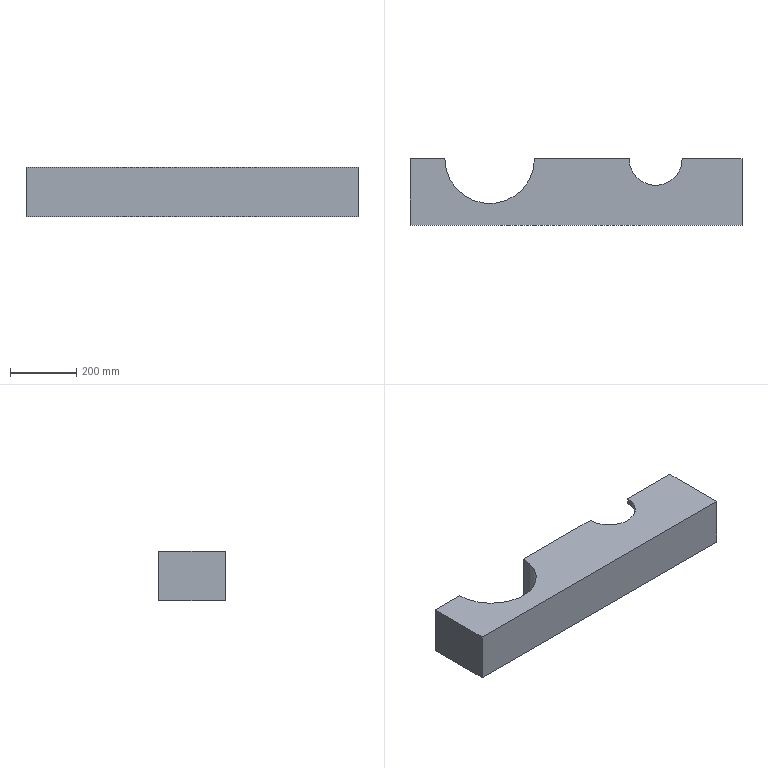Part | SolidWorks | features RefAxis 2, Chamfer 1, Extrusion 1, ICE 1, RevCut 1 | 1 solid | 19 faces | box 1000 x 200 x 150 mm | volume 22425057 mm3 | plane 12 | cylinder 6 | cone 1 | commonest cylinder face diameters 250 x2 160 x1 220 x1 270 x1 280 x1
STEP:
#1=CARTESIAN_POINT('',(660.,0.,150.));
#2=VERTEX_POINT('',#1);
#3=CARTESIAN_POINT('',(660.,0.,132.));
#4=VERTEX_POINT('',#3);
#5=CARTESIAN_POINT('',(660.,0.,0.));
#6=DIRECTION('',(0.,0.,-1.));
#7=VECTOR('',#6,1000.);
#8=LINE('',#5,#7);
#9=EDGE_CURVE('',#2,#4,#8,.T.);
#10=ORIENTED_EDGE('',*,*,#9,.T.);
#11=CARTESIAN_POINT('',(650.,0.,122.));
#12=VERTEX_POINT('',#11);
#13=CARTESIAN_POINT('',(740.,0.,212.));
#14=DIRECTION('',(-0.7071,0.,-0.7071));
#15=VECTOR('',#14,1000.);
#16=LINE('',#13,#15);
#17=EDGE_CURVE('',#4,#12,#16,.T.);
#18=ORIENTED_EDGE('',*,*,#17,.T.);
#19=CARTESIAN_POINT('',(615.,0.,122.));
#20=VERTEX_POINT('',#19);
#21=CARTESIAN_POINT('',(0.,0.,122.));
#22=DIRECTION('',(-1.,0.,0.));
#23=VECTOR('',#22,1000.);
#24=LINE('',#21,#23);
#25=EDGE_CURVE('',#12,#20,#24,.T.);
#26=ORIENTED_EDGE('',*,*,#25,.T.);
#27=CARTESIAN_POINT('',(615.,0.,93.));
#28=VERTEX_POINT('',#27);
#29=CARTESIAN_POINT('',(615.,0.,0.));
#30=DIRECTION('',(0.,0.,-1.));
#31=VECTOR('',#30,1000.);
#32=LINE('',#29,#31);
#33=EDGE_CURVE('',#20,#28,#32,.T.);
#34=ORIENTED_EDGE('',*,*,#33,.T.);
#35=CARTESIAN_POINT('',(600.,0.,93.));
#36=VERTEX_POINT('',#35);
#37=CARTESIAN_POINT('',(0.,0.,93.));
#38=DIRECTION('',(-1.,0.,0.));
#39=VECTOR('',#38,1000.);
#40=LINE('',#37,#39);
#41=EDGE_CURVE('',#28,#36,#40,.T.);
#42=ORIENTED_EDGE('',*,*,#41,.T.);
#43=CARTESIAN_POINT('',(600.,0.,81.));
#44=VERTEX_POINT('',#43);
#45=CARTESIAN_POINT('',(600.,0.,0.));
#46=DIRECTION('',(0.,0.,-1.));
#47=VECTOR('',#46,1000.);
#48=LINE('',#45,#47);
#49=EDGE_CURVE('',#36,#44,#48,.T.);
#50=ORIENTED_EDGE('',*,*,#49,.T.);
#51=CARTESIAN_POINT('',(615.,0.,81.));
#52=VERTEX_POINT('',#51);
#53=CARTESIAN_POINT('',(0.,0.,81.));
#54=DIRECTION('',(1.,0.,0.));
#55=VECTOR('',#54,1000.);
#56=LINE('',#53,#55);
#57=EDGE_CURVE('',#44,#52,#56,.T.);
#58=ORIENTED_EDGE('',*,*,#57,.T.);
#59=CARTESIAN_POINT('',(615.,0.,15.));
#60=VERTEX_POINT('',#59);
#61=CARTESIAN_POINT('',(615.,0.,0.));
#62=DIRECTION('',(0.,0.,-1.));
#63=VECTOR('',#62,1000.);
#64=LINE('',#61,#63);
#65=EDGE_CURVE('',#52,#60,#64,.T.);
#66=ORIENTED_EDGE('',*,*,#65,.T.);
#67=CARTESIAN_POINT('',(630.,0.,15.));
#68=VERTEX_POINT('',#67);
#69=CARTESIAN_POINT('',(0.,0.,15.));
#70=DIRECTION('',(1.,0.,0.));
#71=VECTOR('',#70,1000.);
#72=LINE('',#69,#71);
#73=EDGE_CURVE('',#60,#68,#72,.T.);
#74=ORIENTED_EDGE('',*,*,#73,.T.);
#75=CARTESIAN_POINT('',(630.,0.,0.));
#76=VERTEX_POINT('',#75);
#77=CARTESIAN_POINT('',(630.,0.,0.));
#78=DIRECTION('',(0.,0.,-1.));
#79=VECTOR('',#78,1000.);
#80=LINE('',#77,#79);
#81=EDGE_CURVE('',#68,#76,#80,.T.);
#82=ORIENTED_EDGE('',*,*,#81,.T.);
#83=CARTESIAN_POINT('',(375.,0.,0.));
#84=VERTEX_POINT('',#83);
#85=CARTESIAN_POINT('',(0.,0.,0.));
#86=DIRECTION('',(-1.,0.,0.));
#87=VECTOR('',#86,1000.);
#88=LINE('',#85,#87);
#89=EDGE_CURVE('',#76,#84,#88,.T.);
#90=ORIENTED_EDGE('',*,*,#89,.T.);
#91=CARTESIAN_POINT('',(375.,0.,150.));
#92=VERTEX_POINT('',#91);
#93=CARTESIAN_POINT('',(375.,0.,0.));
#94=DIRECTION('',(0.,0.,1.));
#95=VECTOR('',#94,1000.);
#96=LINE('',#93,#95);
#97=EDGE_CURVE('',#84,#92,#96,.T.);
#98=ORIENTED_EDGE('',*,*,#97,.T.);
#99=CARTESIAN_POINT('',(0.,0.,150.));
#100=DIRECTION('',(-1.,0.,0.));
#101=VECTOR('',#100,1000.);
#102=LINE('',#99,#101);
#103=EDGE_CURVE('',#2,#92,#102,.T.);
#104=ORIENTED_EDGE('',*,*,#103,.F.);
#105=EDGE_LOOP('',(#10,#18,#26,#34,#42,#50,#58,#66,#74,#82,#90,#98,#104));
#106=FACE_OUTER_BOUND('',#105,.T.);
#107=CARTESIAN_POINT('',(0.,0.,150.));
#108=DIRECTION('',(0.,-1.,0.));
#109=DIRECTION('',(0.,0.,-1.));
#110=AXIS2_PLACEMENT_3D('',#107,#108,#109);
#111=PLANE('',#110);
#112=ADVANCED_FACE('',(#106),#111,.F.);
#113=CARTESIAN_POINT('',(865.,0.,122.));
#114=VERTEX_POINT('',#113);
#115=CARTESIAN_POINT('',(830.,0.,122.));
#116=VERTEX_POINT('',#115);
#117=CARTESIAN_POINT('',(0.,0.,122.));
#118=DIRECTION('',(-1.,0.,0.));
#119=VECTOR('',#118,1000.);
#120=LINE('',#117,#119);
#121=EDGE_CURVE('',#114,#116,#120,.T.);
#122=ORIENTED_EDGE('',*,*,#121,.T.);
#123=CARTESIAN_POINT('',(820.,0.,132.));
#124=VERTEX_POINT('',#123);
#125=CARTESIAN_POINT('',(740.,0.,212.));
#126=DIRECTION('',(-0.7071,0.,0.7071));
#127=VECTOR('',#126,1000.);
#128=LINE('',#125,#127);
#129=EDGE_CURVE('',#116,#124,#128,.T.);
#130=ORIENTED_EDGE('',*,*,#129,.T.);
#131=CARTESIAN_POINT('',(820.,0.,150.));
#132=VERTEX_POINT('',#131);
#133=CARTESIAN_POINT('',(820.,0.,0.));
#134=DIRECTION('',(0.,0.,1.));
#135=VECTOR('',#134,1000.);
#136=LINE('',#133,#135);
#137=EDGE_CURVE('',#124,#132,#136,.T.);
#138=ORIENTED_EDGE('',*,*,#137,.T.);
#139=CARTESIAN_POINT('',(1000.,0.,150.));
#140=VERTEX_POINT('',#139);
#141=CARTESIAN_POINT('',(0.,0.,150.));
#142=DIRECTION('',(-1.,0.,0.));
#143=VECTOR('',#142,1000.);
#144=LINE('',#141,#143);
#145=EDGE_CURVE('',#140,#132,#144,.T.);
#146=ORIENTED_EDGE('',*,*,#145,.F.);
#147=CARTESIAN_POINT('',(1000.,0.,0.));
#148=VERTEX_POINT('',#147);
#149=CARTESIAN_POINT('',(1000.,0.,150.));
#150=DIRECTION('',(0.,0.,-1.));
#151=VECTOR('',#150,1000.);
#152=LINE('',#149,#151);
#153=EDGE_CURVE('',#140,#148,#152,.T.);
#154=ORIENTED_EDGE('',*,*,#153,.T.);
#155=CARTESIAN_POINT('',(850.,0.,0.));
#156=VERTEX_POINT('',#155);
#157=CARTESIAN_POINT('',(0.,0.,0.));
#158=DIRECTION('',(-1.,0.,0.));
#159=VECTOR('',#158,1000.);
#160=LINE('',#157,#159);
#161=EDGE_CURVE('',#148,#156,#160,.T.);
#162=ORIENTED_EDGE('',*,*,#161,.T.);
#163=CARTESIAN_POINT('',(850.,0.,15.));
#164=VERTEX_POINT('',#163);
#165=CARTESIAN_POINT('',(850.,0.,0.));
#166=DIRECTION('',(0.,0.,1.));
#167=VECTOR('',#166,1000.);
#168=LINE('',#165,#167);
#169=EDGE_CURVE('',#156,#164,#168,.T.);
#170=ORIENTED_EDGE('',*,*,#169,.T.);
#171=CARTESIAN_POINT('',(865.,0.,15.));
#172=VERTEX_POINT('',#171);
#173=CARTESIAN_POINT('',(0.,0.,15.));
#174=DIRECTION('',(1.,0.,0.));
#175=VECTOR('',#174,1000.);
#176=LINE('',#173,#175);
#177=EDGE_CURVE('',#164,#172,#176,.T.);
#178=ORIENTED_EDGE('',*,*,#177,.T.);
#179=CARTESIAN_POINT('',(865.,0.,81.));
#180=VERTEX_POINT('',#179);
#181=CARTESIAN_POINT('',(865.,0.,0.));
#182=DIRECTION('',(0.,0.,1.));
#183=VECTOR('',#182,1000.);
#184=LINE('',#181,#183);
#185=EDGE_CURVE('',#172,#180,#184,.T.);
#186=ORIENTED_EDGE('',*,*,#185,.T.);
#187=CARTESIAN_POINT('',(880.,0.,81.));
#188=VERTEX_POINT('',#187);
#189=CARTESIAN_POINT('',(0.,0.,81.));
#190=DIRECTION('',(1.,0.,0.));
#191=VECTOR('',#190,1000.);
#192=LINE('',#189,#191);
#193=EDGE_CURVE('',#180,#188,#192,.T.);
#194=ORIENTED_EDGE('',*,*,#193,.T.);
#195=CARTESIAN_POINT('',(880.,0.,93.));
#196=VERTEX_POINT('',#195);
#197=CARTESIAN_POINT('',(880.,0.,0.));
#198=DIRECTION('',(0.,0.,1.));
#199=VECTOR('',#198,1000.);
#200=LINE('',#197,#199);
#201=EDGE_CURVE('',#188,#196,#200,.T.);
#202=ORIENTED_EDGE('',*,*,#201,.T.);
#203=CARTESIAN_POINT('',(865.,0.,93.));
#204=VERTEX_POINT('',#203);
#205=CARTESIAN_POINT('',(0.,0.,93.));
#206=DIRECTION('',(-1.,0.,0.));
#207=VECTOR('',#206,1000.);
#208=LINE('',#205,#207);
#209=EDGE_CURVE('',#196,#204,#208,.T.);
#210=ORIENTED_EDGE('',*,*,#209,.T.);
#211=CARTESIAN_POINT('',(865.,0.,0.));
#212=DIRECTION('',(0.,0.,1.));
#213=VECTOR('',#212,1000.);
#214=LINE('',#211,#213);
#215=EDGE_CURVE('',#204,#114,#214,.T.);
#216=ORIENTED_EDGE('',*,*,#215,.T.);
#217=EDGE_LOOP('',(#122,#130,#138,#146,#154,#162,#170,#178,#186,#194,#202,#210,#216));
#218=FACE_OUTER_BOUND('',#217,.T.);
#219=CARTESIAN_POINT('',(0.,0.,150.));
#220=DIRECTION('',(0.,-1.,0.));
#221=DIRECTION('',(0.,0.,-1.));
#222=AXIS2_PLACEMENT_3D('',#219,#220,#221);
#223=PLANE('',#222);
#224=ADVANCED_FACE('',(#218),#223,.F.);
#225=CARTESIAN_POINT('',(0.,0.,0.));
#226=VERTEX_POINT('',#225);
#227=CARTESIAN_POINT('',(0.,-200.,0.));
#228=VERTEX_POINT('',#227);
#229=CARTESIAN_POINT('',(0.,0.,0.));
#230=DIRECTION('',(0.,-1.,0.));
#231=VECTOR('',#230,1000.);
#232=LINE('',#229,#231);
#233=EDGE_CURVE('',#226,#228,#232,.T.);
#234=ORIENTED_EDGE('',*,*,#233,.T.);
#235=CARTESIAN_POINT('',(0.,-200.,150.));
#236=VERTEX_POINT('',#235);
#237=CARTESIAN_POINT('',(0.,-200.,150.));
#238=DIRECTION('',(0.,0.,-1.));
#239=VECTOR('',#238,1000.);
#240=LINE('',#237,#239);
#241=EDGE_CURVE('',#236,#228,#240,.T.);
#242=ORIENTED_EDGE('',*,*,#241,.F.);
#243=CARTESIAN_POINT('',(0.,0.,150.));
#244=VERTEX_POINT('',#243);
#245=CARTESIAN_POINT('',(0.,0.,150.));
#246=DIRECTION('',(0.,-1.,0.));
#247=VECTOR('',#246,1000.);
#248=LINE('',#245,#247);
#249=EDGE_CURVE('',#244,#236,#248,.T.);
#250=ORIENTED_EDGE('',*,*,#249,.F.);
#251=CARTESIAN_POINT('',(0.,0.,150.));
#252=DIRECTION('',(0.,0.,-1.));
#253=VECTOR('',#252,1000.);
#254=LINE('',#251,#253);
#255=EDGE_CURVE('',#244,#226,#254,.T.);
#256=ORIENTED_EDGE('',*,*,#255,.T.);
#257=EDGE_LOOP('',(#234,#242,#250,#256));
#258=FACE_OUTER_BOUND('',#257,.T.);
#259=CARTESIAN_POINT('',(0.,0.,150.));
#260=DIRECTION('',(1.,0.,0.));
#261=DIRECTION('',(0.,0.,-1.));
#262=AXIS2_PLACEMENT_3D('',#259,#260,#261);
#263=PLANE('',#262);
#264=ADVANCED_FACE('',(#258),#263,.F.);
#265=CARTESIAN_POINT('',(1000.,-200.,0.));
#266=VERTEX_POINT('',#265);
#267=CARTESIAN_POINT('',(0.,-200.,0.));
#268=DIRECTION('',(1.,0.,0.));
#269=VECTOR('',#268,1000.);
#270=LINE('',#267,#269);
#271=EDGE_CURVE('',#228,#266,#270,.T.);
#272=ORIENTED_EDGE('',*,*,#271,.T.);
#273=CARTESIAN_POINT('',(1000.,-200.,150.));
#274=VERTEX_POINT('',#273);
#275=CARTESIAN_POINT('',(1000.,-200.,150.));
#276=DIRECTION('',(0.,0.,-1.));
#277=VECTOR('',#276,1000.);
#278=LINE('',#275,#277);
#279=EDGE_CURVE('',#274,#266,#278,.T.);
#280=ORIENTED_EDGE('',*,*,#279,.F.);
#281=CARTESIAN_POINT('',(0.,-200.,150.));
#282=DIRECTION('',(1.,0.,0.));
#283=VECTOR('',#282,1000.);
#284=LINE('',#281,#283);
#285=EDGE_CURVE('',#236,#274,#284,.T.);
#286=ORIENTED_EDGE('',*,*,#285,.F.);
#287=ORIENTED_EDGE('',*,*,#241,.T.);
#288=EDGE_LOOP('',(#272,#280,#286,#287));
#289=FACE_OUTER_BOUND('',#288,.T.);
#290=CARTESIAN_POINT('',(0.,-200.,150.));
#291=DIRECTION('',(0.,1.,0.));
#292=DIRECTION('',(0.,0.,1.));
#293=AXIS2_PLACEMENT_3D('',#290,#291,#292);
#294=PLANE('',#293);
#295=ADVANCED_FACE('',(#289),#294,.F.);
#296=CARTESIAN_POINT('',(1000.,0.,0.));
#297=DIRECTION('',(0.,1.,0.));
#298=VECTOR('',#297,1000.);
#299=LINE('',#296,#298);
#300=EDGE_CURVE('',#266,#148,#299,.T.);
#301=ORIENTED_EDGE('',*,*,#300,.T.);
#302=ORIENTED_EDGE('',*,*,#153,.F.);
#303=CARTESIAN_POINT('',(1000.,0.,150.));
#304=DIRECTION('',(0.,1.,0.));
#305=VECTOR('',#304,1000.);
#306=LINE('',#303,#305);
#307=EDGE_CURVE('',#274,#140,#306,.T.);
#308=ORIENTED_EDGE('',*,*,#307,.F.);
#309=ORIENTED_EDGE('',*,*,#279,.T.);
#310=EDGE_LOOP('',(#301,#302,#308,#309));
#311=FACE_OUTER_BOUND('',#310,.T.);
#312=CARTESIAN_POINT('',(1000.,0.,150.));
#313=DIRECTION('',(-1.,0.,0.));
#314=DIRECTION('',(0.,0.,1.));
#315=AXIS2_PLACEMENT_3D('',#312,#313,#314);
#316=PLANE('',#315);
#317=ADVANCED_FACE('',(#311),#316,.F.);
#318=CARTESIAN_POINT('',(105.,0.,150.));
#319=VERTEX_POINT('',#318);
#320=CARTESIAN_POINT('',(0.,0.,150.));
#321=DIRECTION('',(-1.,0.,0.));
#322=VECTOR('',#321,1000.);
#323=LINE('',#320,#322);
#324=EDGE_CURVE('',#319,#244,#323,.T.);
#325=ORIENTED_EDGE('',*,*,#324,.F.);
#326=CARTESIAN_POINT('',(105.,0.,0.));
#327=VERTEX_POINT('',#326);
#328=CARTESIAN_POINT('',(105.,0.,0.));
#329=DIRECTION('',(0.,0.,-1.));
#330=VECTOR('',#329,1000.);
#331=LINE('',#328,#330);
#332=EDGE_CURVE('',#319,#327,#331,.T.);
#333=ORIENTED_EDGE('',*,*,#332,.T.);
#334=CARTESIAN_POINT('',(0.,0.,0.));
#335=DIRECTION('',(-1.,0.,0.));
#336=VECTOR('',#335,1000.);
#337=LINE('',#334,#336);
#338=EDGE_CURVE('',#327,#226,#337,.T.);
#339=ORIENTED_EDGE('',*,*,#338,.T.);
#340=ORIENTED_EDGE('',*,*,#255,.F.);
#341=EDGE_LOOP('',(#325,#333,#339,#340));
#342=FACE_OUTER_BOUND('',#341,.T.);
#343=CARTESIAN_POINT('',(0.,0.,150.));
#344=DIRECTION('',(0.,-1.,0.));
#345=DIRECTION('',(0.,0.,-1.));
#346=AXIS2_PLACEMENT_3D('',#343,#344,#345);
#347=PLANE('',#346);
#348=ADVANCED_FACE('',(#342),#347,.F.);
#349=CARTESIAN_POINT('',(240.,0.,150.));
#350=DIRECTION('',(0.,0.,1.));
#351=DIRECTION('',(1.,0.,0.));
#352=AXIS2_PLACEMENT_3D('',#349,#350,#351);
#353=CIRCLE('',#352,135.);
#354=EDGE_CURVE('',#319,#92,#353,.T.);
#355=ORIENTED_EDGE('',*,*,#354,.F.);
#356=ORIENTED_EDGE('',*,*,#324,.T.);
#357=ORIENTED_EDGE('',*,*,#249,.T.);
#358=ORIENTED_EDGE('',*,*,#285,.T.);
#359=ORIENTED_EDGE('',*,*,#307,.T.);
#360=ORIENTED_EDGE('',*,*,#145,.T.);
#361=CARTESIAN_POINT('',(740.,0.,150.));
#362=DIRECTION('',(0.,0.,1.));
#363=DIRECTION('',(1.,0.,0.));
#364=AXIS2_PLACEMENT_3D('',#361,#362,#363);
#365=CIRCLE('',#364,80.);
#366=EDGE_CURVE('',#2,#132,#365,.T.);
#367=ORIENTED_EDGE('',*,*,#366,.F.);
#368=ORIENTED_EDGE('',*,*,#103,.T.);
#369=EDGE_LOOP('',(#355,#356,#357,#358,#359,#360,#367,#368));
#370=FACE_OUTER_BOUND('',#369,.T.);
#371=CARTESIAN_POINT('',(0.,0.,150.));
#372=DIRECTION('',(0.,0.,1.));
#373=DIRECTION('',(1.,0.,0.));
#374=AXIS2_PLACEMENT_3D('',#371,#372,#373);
#375=PLANE('',#374);
#376=ADVANCED_FACE('',(#370),#375,.T.);
#377=ORIENTED_EDGE('',*,*,#89,.F.);
#378=CARTESIAN_POINT('',(740.,0.,0.));
#379=DIRECTION('',(0.,0.,-1.));
#380=DIRECTION('',(-1.,0.,0.));
#381=AXIS2_PLACEMENT_3D('',#378,#379,#380);
#382=CIRCLE('',#381,110.);
#383=EDGE_CURVE('',#156,#76,#382,.T.);
#384=ORIENTED_EDGE('',*,*,#383,.F.);
#385=ORIENTED_EDGE('',*,*,#161,.F.);
#386=ORIENTED_EDGE('',*,*,#300,.F.);
#387=ORIENTED_EDGE('',*,*,#271,.F.);
#388=ORIENTED_EDGE('',*,*,#233,.F.);
#389=ORIENTED_EDGE('',*,*,#338,.F.);
#390=CARTESIAN_POINT('',(240.,0.,0.));
#391=DIRECTION('',(0.,0.,1.));
#392=DIRECTION('',(1.,0.,0.));
#393=AXIS2_PLACEMENT_3D('',#390,#391,#392);
#394=CIRCLE('',#393,135.);
#395=EDGE_CURVE('',#327,#84,#394,.T.);
#396=ORIENTED_EDGE('',*,*,#395,.T.);
#397=EDGE_LOOP('',(#377,#384,#385,#386,#387,#388,#389,#396));
#398=FACE_OUTER_BOUND('',#397,.T.);
#399=CARTESIAN_POINT('',(0.,0.,0.));
#400=DIRECTION('',(0.,0.,1.));
#401=DIRECTION('',(1.,0.,0.));
#402=AXIS2_PLACEMENT_3D('',#399,#400,#401);
#403=PLANE('',#402);
#404=ADVANCED_FACE('',(#398),#403,.F.);
#405=ORIENTED_EDGE('',*,*,#137,.F.);
#406=CARTESIAN_POINT('',(740.,0.,132.));
#407=DIRECTION('',(0.,0.,-1.));
#408=DIRECTION('',(1.,0.,0.));
#409=AXIS2_PLACEMENT_3D('',#406,#407,#408);
#410=CIRCLE('',#409,80.);
#411=EDGE_CURVE('',#124,#4,#410,.T.);
#412=ORIENTED_EDGE('',*,*,#411,.T.);
#413=ORIENTED_EDGE('',*,*,#9,.F.);
#414=ORIENTED_EDGE('',*,*,#366,.T.);
#415=EDGE_LOOP('',(#405,#412,#413,#414));
#416=FACE_OUTER_BOUND('',#415,.T.);
#417=CARTESIAN_POINT('',(740.,0.,0.));
#418=DIRECTION('',(0.,0.,1.));
#419=DIRECTION('',(1.,0.,0.));
#420=AXIS2_PLACEMENT_3D('',#417,#418,#419);
#421=CYLINDRICAL_SURFACE('',#420,80.);
#422=ADVANCED_FACE('',(#416),#421,.F.);
#423=ORIENTED_EDGE('',*,*,#395,.F.);
#424=ORIENTED_EDGE('',*,*,#332,.F.);
#425=ORIENTED_EDGE('',*,*,#354,.T.);
#426=ORIENTED_EDGE('',*,*,#97,.F.);
#427=EDGE_LOOP('',(#423,#424,#425,#426));
#428=FACE_OUTER_BOUND('',#427,.T.);
#429=CARTESIAN_POINT('',(240.,0.,0.));
#430=DIRECTION('',(0.,0.,1.));
#431=DIRECTION('',(1.,0.,0.));
#432=AXIS2_PLACEMENT_3D('',#429,#430,#431);
#433=CYLINDRICAL_SURFACE('',#432,135.);
#434=ADVANCED_FACE('',(#428),#433,.F.);
#435=CARTESIAN_POINT('',(740.,0.,122.));
#436=DIRECTION('',(0.,0.,-1.));
#437=DIRECTION('',(-1.,0.,0.));
#438=AXIS2_PLACEMENT_3D('',#435,#436,#437);
#439=CIRCLE('',#438,125.);
#440=EDGE_CURVE('',#114,#20,#439,.T.);
#441=ORIENTED_EDGE('',*,*,#440,.F.);
#442=ORIENTED_EDGE('',*,*,#215,.F.);
#443=CARTESIAN_POINT('',(740.,0.,93.));
#444=DIRECTION('',(0.,0.,-1.));
#445=DIRECTION('',(-1.,0.,0.));
#446=AXIS2_PLACEMENT_3D('',#443,#444,#445);
#447=CIRCLE('',#446,125.);
#448=EDGE_CURVE('',#204,#28,#447,.T.);
#449=ORIENTED_EDGE('',*,*,#448,.T.);
#450=ORIENTED_EDGE('',*,*,#33,.F.);
#451=EDGE_LOOP('',(#441,#442,#449,#450));
#452=FACE_OUTER_BOUND('',#451,.T.);
#453=CARTESIAN_POINT('',(740.,0.,0.));
#454=DIRECTION('',(0.,0.,-1.));
#455=DIRECTION('',(-1.,0.,0.));
#456=AXIS2_PLACEMENT_3D('',#453,#454,#455);
#457=CYLINDRICAL_SURFACE('',#456,125.);
#458=ADVANCED_FACE('',(#452),#457,.F.);
#459=ORIENTED_EDGE('',*,*,#448,.F.);
#460=ORIENTED_EDGE('',*,*,#209,.F.);
#461=CARTESIAN_POINT('',(740.,0.,93.));
#462=DIRECTION('',(0.,0.,-1.));
#463=DIRECTION('',(-1.,0.,0.));
#464=AXIS2_PLACEMENT_3D('',#461,#462,#463);
#465=CIRCLE('',#464,140.);
#466=EDGE_CURVE('',#196,#36,#465,.T.);
#467=ORIENTED_EDGE('',*,*,#466,.T.);
#468=ORIENTED_EDGE('',*,*,#41,.F.);
#469=EDGE_LOOP('',(#459,#460,#467,#468));
#470=FACE_OUTER_BOUND('',#469,.T.);
#471=CARTESIAN_POINT('',(600.,0.,93.));
#472=DIRECTION('',(0.,0.,1.));
#473=DIRECTION('',(1.,0.,0.));
#474=AXIS2_PLACEMENT_3D('',#471,#472,#473);
#475=PLANE('',#474);
#476=ADVANCED_FACE('',(#470),#475,.F.);
#477=ORIENTED_EDGE('',*,*,#466,.F.);
#478=ORIENTED_EDGE('',*,*,#201,.F.);
#479=CARTESIAN_POINT('',(740.,0.,81.));
#480=DIRECTION('',(0.,0.,-1.));
#481=DIRECTION('',(-1.,0.,0.));
#482=AXIS2_PLACEMENT_3D('',#479,#480,#481);
#483=CIRCLE('',#482,140.);
#484=EDGE_CURVE('',#188,#44,#483,.T.);
#485=ORIENTED_EDGE('',*,*,#484,.T.);
#486=ORIENTED_EDGE('',*,*,#49,.F.);
#487=EDGE_LOOP('',(#477,#478,#485,#486));
#488=FACE_OUTER_BOUND('',#487,.T.);
#489=CARTESIAN_POINT('',(740.,0.,0.));
#490=DIRECTION('',(0.,0.,-1.));
#491=DIRECTION('',(-1.,0.,0.));
#492=AXIS2_PLACEMENT_3D('',#489,#490,#491);
#493=CYLINDRICAL_SURFACE('',#492,140.);
#494=ADVANCED_FACE('',(#488),#493,.F.);
#495=ORIENTED_EDGE('',*,*,#484,.F.);
#496=ORIENTED_EDGE('',*,*,#193,.F.);
#497=CARTESIAN_POINT('',(740.,0.,81.));
#498=DIRECTION('',(0.,0.,-1.));
#499=DIRECTION('',(-1.,0.,0.));
#500=AXIS2_PLACEMENT_3D('',#497,#498,#499);
#501=CIRCLE('',#500,125.);
#502=EDGE_CURVE('',#180,#52,#501,.T.);
#503=ORIENTED_EDGE('',*,*,#502,.T.);
#504=ORIENTED_EDGE('',*,*,#57,.F.);
#505=EDGE_LOOP('',(#495,#496,#503,#504));
#506=FACE_OUTER_BOUND('',#505,.T.);
#507=CARTESIAN_POINT('',(615.,0.,81.));
#508=DIRECTION('',(0.,0.,-1.));
#509=DIRECTION('',(-1.,0.,0.));
#510=AXIS2_PLACEMENT_3D('',#507,#508,#509);
#511=PLANE('',#510);
#512=ADVANCED_FACE('',(#506),#511,.F.);
#513=ORIENTED_EDGE('',*,*,#502,.F.);
#514=ORIENTED_EDGE('',*,*,#185,.F.);
#515=CARTESIAN_POINT('',(740.,0.,15.));
#516=DIRECTION('',(0.,0.,-1.));
#517=DIRECTION('',(-1.,0.,0.));
#518=AXIS2_PLACEMENT_3D('',#515,#516,#517);
#519=CIRCLE('',#518,125.);
#520=EDGE_CURVE('',#172,#60,#519,.T.);
#521=ORIENTED_EDGE('',*,*,#520,.T.);
#522=ORIENTED_EDGE('',*,*,#65,.F.);
#523=EDGE_LOOP('',(#513,#514,#521,#522));
#524=FACE_OUTER_BOUND('',#523,.T.);
#525=CARTESIAN_POINT('',(740.,0.,0.));
#526=DIRECTION('',(0.,0.,-1.));
#527=DIRECTION('',(-1.,0.,0.));
#528=AXIS2_PLACEMENT_3D('',#525,#526,#527);
#529=CYLINDRICAL_SURFACE('',#528,125.);
#530=ADVANCED_FACE('',(#524),#529,.F.);
#531=ORIENTED_EDGE('',*,*,#520,.F.);
#532=ORIENTED_EDGE('',*,*,#177,.F.);
#533=CARTESIAN_POINT('',(740.,0.,15.));
#534=DIRECTION('',(0.,0.,-1.));
#535=DIRECTION('',(-1.,0.,0.));
#536=AXIS2_PLACEMENT_3D('',#533,#534,#535);
#537=CIRCLE('',#536,110.);
#538=EDGE_CURVE('',#164,#68,#537,.T.);
#539=ORIENTED_EDGE('',*,*,#538,.T.);
#540=ORIENTED_EDGE('',*,*,#73,.F.);
#541=EDGE_LOOP('',(#531,#532,#539,#540));
#542=FACE_OUTER_BOUND('',#541,.T.);
#543=CARTESIAN_POINT('',(630.,0.,15.));
#544=DIRECTION('',(0.,0.,-1.));
#545=DIRECTION('',(-1.,0.,0.));
#546=AXIS2_PLACEMENT_3D('',#543,#544,#545);
#547=PLANE('',#546);
#548=ADVANCED_FACE('',(#542),#547,.F.);
#549=ORIENTED_EDGE('',*,*,#538,.F.);
#550=ORIENTED_EDGE('',*,*,#169,.F.);
#551=ORIENTED_EDGE('',*,*,#383,.T.);
#552=ORIENTED_EDGE('',*,*,#81,.F.);
#553=EDGE_LOOP('',(#549,#550,#551,#552));
#554=FACE_OUTER_BOUND('',#553,.T.);
#555=CARTESIAN_POINT('',(740.,0.,0.));
#556=DIRECTION('',(0.,0.,-1.));
#557=DIRECTION('',(-1.,0.,0.));
#558=AXIS2_PLACEMENT_3D('',#555,#556,#557);
#559=CYLINDRICAL_SURFACE('',#558,110.);
#560=ADVANCED_FACE('',(#554),#559,.F.);
#561=ORIENTED_EDGE('',*,*,#25,.F.);
#562=CARTESIAN_POINT('',(740.,0.,122.));
#563=DIRECTION('',(0.,0.,1.));
#564=DIRECTION('',(1.,0.,0.));
#565=AXIS2_PLACEMENT_3D('',#562,#563,#564);
#566=CIRCLE('',#565,90.);
#567=EDGE_CURVE('',#12,#116,#566,.T.);
#568=ORIENTED_EDGE('',*,*,#567,.T.);
#569=ORIENTED_EDGE('',*,*,#121,.F.);
#570=ORIENTED_EDGE('',*,*,#440,.T.);
#571=EDGE_LOOP('',(#561,#568,#569,#570));
#572=FACE_OUTER_BOUND('',#571,.T.);
#573=CARTESIAN_POINT('',(615.,0.,122.));
#574=DIRECTION('',(0.,0.,1.));
#575=DIRECTION('',(1.,0.,0.));
#576=AXIS2_PLACEMENT_3D('',#573,#574,#575);
#577=PLANE('',#576);
#578=ADVANCED_FACE('',(#572),#577,.F.);
#579=ORIENTED_EDGE('',*,*,#129,.F.);
#580=ORIENTED_EDGE('',*,*,#567,.F.);
#581=ORIENTED_EDGE('',*,*,#17,.F.);
#582=ORIENTED_EDGE('',*,*,#411,.F.);
#583=EDGE_LOOP('',(#579,#580,#581,#582));
#584=FACE_OUTER_BOUND('',#583,.T.);
#585=CARTESIAN_POINT('',(740.,0.,132.));
#586=DIRECTION('',(0.,0.,-1.));
#587=DIRECTION('',(-1.,0.,0.));
#588=AXIS2_PLACEMENT_3D('',#585,#586,#587);
#589=CONICAL_SURFACE('',#588,80.,0.7854);
#590=ADVANCED_FACE('',(#584),#589,.F.);
#591=CLOSED_SHELL('',(#112,#224,#264,#295,#317,#348,#376,#404,#422,#434,#458,#476,#494,#512,#530,#548,#560,#578,#590));
#592=MANIFOLD_SOLID_BREP('',#591);
#593=CARTESIAN_POINT('',(0.,0.,0.));
#594=DIRECTION('',(0.,0.,1.));
#595=DIRECTION('',(1.,0.,0.));
#596=AXIS2_PLACEMENT_3D('',#593,#594,#595);
#597=(LENGTH_UNIT()NAMED_UNIT(*)SI_UNIT(.MILLI.,.METRE.));
#598=UNCERTAINTY_MEASURE_WITH_UNIT(LENGTH_MEASURE(0.00001),#597,'','');
#599=(NAMED_UNIT(*)PLANE_ANGLE_UNIT()SI_UNIT($,.RADIAN.));
#600=(NAMED_UNIT(*)SI_UNIT($,.STERADIAN.)SOLID_ANGLE_UNIT());
#601=(GEOMETRIC_REPRESENTATION_CONTEXT(3)GLOBAL_UNCERTAINTY_ASSIGNED_CONTEXT((#598))GLOBAL_UNIT_ASSIGNED_CONTEXT((#597,#599,#600))REPRESENTATION_CONTEXT('',''));
#602=ADVANCED_BREP_SHAPE_REPRESENTATION('',(#592,#596),#601);